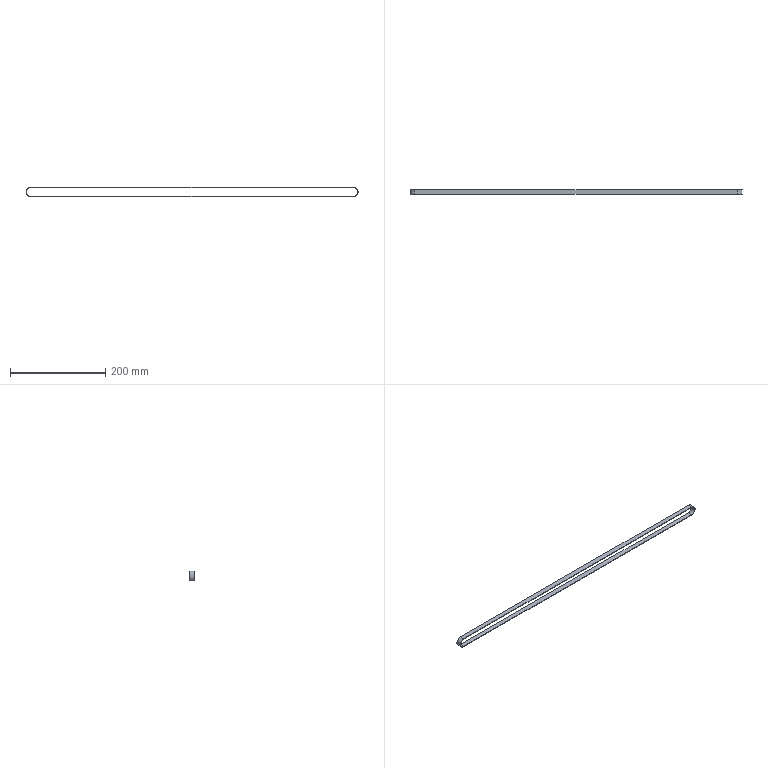Part | SolidWorks | features BaseBody 1 | 1 solid | 10 faces | box 695.6 x 10 x 20.6 mm | volume 16931 mm3 | plane 6 | cylinder 4 | commonest cylinder face diameters 18.2 x2 20.6 x2
STEP:
#1=CARTESIAN_POINT('',(675.,0.,-9.1));
#2=VERTEX_POINT('',#1);
#3=CARTESIAN_POINT('',(0.,0.,-9.1));
#4=VERTEX_POINT('',#3);
#5=CARTESIAN_POINT('',(675.,0.,-9.1));
#6=DIRECTION('',(-1.,0.,0.));
#7=VECTOR('',#6,1000.);
#8=LINE('',#5,#7);
#9=EDGE_CURVE('',#2,#4,#8,.T.);
#10=ORIENTED_EDGE('',*,*,#9,.F.);
#11=CARTESIAN_POINT('',(675.,10.,-9.1));
#12=VERTEX_POINT('',#11);
#13=CARTESIAN_POINT('',(675.,10.,-9.1));
#14=DIRECTION('',(0.,-1.,0.));
#15=VECTOR('',#14,1000.);
#16=LINE('',#13,#15);
#17=EDGE_CURVE('',#12,#2,#16,.T.);
#18=ORIENTED_EDGE('',*,*,#17,.F.);
#19=CARTESIAN_POINT('',(0.,10.,-9.1));
#20=VERTEX_POINT('',#19);
#21=CARTESIAN_POINT('',(675.,10.,-9.1));
#22=DIRECTION('',(-1.,0.,0.));
#23=VECTOR('',#22,1000.);
#24=LINE('',#21,#23);
#25=EDGE_CURVE('',#12,#20,#24,.T.);
#26=ORIENTED_EDGE('',*,*,#25,.T.);
#27=CARTESIAN_POINT('',(0.,10.,-9.1));
#28=DIRECTION('',(0.,-1.,0.));
#29=VECTOR('',#28,1000.);
#30=LINE('',#27,#29);
#31=EDGE_CURVE('',#20,#4,#30,.T.);
#32=ORIENTED_EDGE('',*,*,#31,.T.);
#33=EDGE_LOOP('',(#10,#18,#26,#32));
#34=FACE_OUTER_BOUND('',#33,.T.);
#35=CARTESIAN_POINT('',(675.,10.,-9.1));
#36=DIRECTION('',(0.,0.,1.));
#37=DIRECTION('',(1.,0.,0.));
#38=AXIS2_PLACEMENT_3D('',#35,#36,#37);
#39=PLANE('',#38);
#40=ADVANCED_FACE('',(#34),#39,.T.);
#41=CARTESIAN_POINT('',(675.,0.,9.1));
#42=VERTEX_POINT('',#41);
#43=CARTESIAN_POINT('',(675.,0.,0.));
#44=DIRECTION('',(0.,1.,0.));
#45=DIRECTION('',(0.,0.,1.));
#46=AXIS2_PLACEMENT_3D('',#43,#44,#45);
#47=CIRCLE('',#46,9.1);
#48=EDGE_CURVE('',#42,#2,#47,.T.);
#49=ORIENTED_EDGE('',*,*,#48,.F.);
#50=CARTESIAN_POINT('',(675.,10.,9.1));
#51=VERTEX_POINT('',#50);
#52=CARTESIAN_POINT('',(675.,10.,9.1));
#53=DIRECTION('',(0.,-1.,0.));
#54=VECTOR('',#53,1000.);
#55=LINE('',#52,#54);
#56=EDGE_CURVE('',#51,#42,#55,.T.);
#57=ORIENTED_EDGE('',*,*,#56,.F.);
#58=CARTESIAN_POINT('',(675.,10.,0.));
#59=DIRECTION('',(0.,1.,0.));
#60=DIRECTION('',(0.,0.,1.));
#61=AXIS2_PLACEMENT_3D('',#58,#59,#60);
#62=CIRCLE('',#61,9.1);
#63=EDGE_CURVE('',#51,#12,#62,.T.);
#64=ORIENTED_EDGE('',*,*,#63,.T.);
#65=ORIENTED_EDGE('',*,*,#17,.T.);
#66=EDGE_LOOP('',(#49,#57,#64,#65));
#67=FACE_OUTER_BOUND('',#66,.T.);
#68=CARTESIAN_POINT('',(675.,10.,0.));
#69=DIRECTION('',(0.,-1.,0.));
#70=DIRECTION('',(0.,0.,-1.));
#71=AXIS2_PLACEMENT_3D('',#68,#69,#70);
#72=CYLINDRICAL_SURFACE('',#71,9.1);
#73=ADVANCED_FACE('',(#67),#72,.F.);
#74=CARTESIAN_POINT('',(0.,0.,9.1));
#75=VERTEX_POINT('',#74);
#76=CARTESIAN_POINT('',(0.,0.,9.1));
#77=DIRECTION('',(1.,0.,0.));
#78=VECTOR('',#77,1000.);
#79=LINE('',#76,#78);
#80=EDGE_CURVE('',#75,#42,#79,.T.);
#81=ORIENTED_EDGE('',*,*,#80,.F.);
#82=CARTESIAN_POINT('',(0.,10.,9.1));
#83=VERTEX_POINT('',#82);
#84=CARTESIAN_POINT('',(0.,10.,9.1));
#85=DIRECTION('',(0.,-1.,0.));
#86=VECTOR('',#85,1000.);
#87=LINE('',#84,#86);
#88=EDGE_CURVE('',#83,#75,#87,.T.);
#89=ORIENTED_EDGE('',*,*,#88,.F.);
#90=CARTESIAN_POINT('',(0.,10.,9.1));
#91=DIRECTION('',(1.,0.,0.));
#92=VECTOR('',#91,1000.);
#93=LINE('',#90,#92);
#94=EDGE_CURVE('',#83,#51,#93,.T.);
#95=ORIENTED_EDGE('',*,*,#94,.T.);
#96=ORIENTED_EDGE('',*,*,#56,.T.);
#97=EDGE_LOOP('',(#81,#89,#95,#96));
#98=FACE_OUTER_BOUND('',#97,.T.);
#99=CARTESIAN_POINT('',(0.,10.,9.1));
#100=DIRECTION('',(0.,0.,-1.));
#101=DIRECTION('',(0.,-1.,0.));
#102=AXIS2_PLACEMENT_3D('',#99,#100,#101);
#103=PLANE('',#102);
#104=ADVANCED_FACE('',(#98),#103,.T.);
#105=CARTESIAN_POINT('',(0.,0.,0.));
#106=DIRECTION('',(0.,1.,0.));
#107=DIRECTION('',(0.,0.,1.));
#108=AXIS2_PLACEMENT_3D('',#105,#106,#107);
#109=CIRCLE('',#108,9.1);
#110=EDGE_CURVE('',#4,#75,#109,.T.);
#111=ORIENTED_EDGE('',*,*,#110,.F.);
#112=ORIENTED_EDGE('',*,*,#31,.F.);
#113=CARTESIAN_POINT('',(0.,10.,0.));
#114=DIRECTION('',(0.,1.,0.));
#115=DIRECTION('',(0.,0.,1.));
#116=AXIS2_PLACEMENT_3D('',#113,#114,#115);
#117=CIRCLE('',#116,9.1);
#118=EDGE_CURVE('',#20,#83,#117,.T.);
#119=ORIENTED_EDGE('',*,*,#118,.T.);
#120=ORIENTED_EDGE('',*,*,#88,.T.);
#121=EDGE_LOOP('',(#111,#112,#119,#120));
#122=FACE_OUTER_BOUND('',#121,.T.);
#123=CARTESIAN_POINT('',(0.,10.,0.));
#124=DIRECTION('',(0.,-1.,0.));
#125=DIRECTION('',(0.,0.,-1.));
#126=AXIS2_PLACEMENT_3D('',#123,#124,#125);
#127=CYLINDRICAL_SURFACE('',#126,9.1);
#128=ADVANCED_FACE('',(#122),#127,.F.);
#129=CARTESIAN_POINT('',(675.,0.,-10.3));
#130=VERTEX_POINT('',#129);
#131=CARTESIAN_POINT('',(0.,0.,-10.3));
#132=VERTEX_POINT('',#131);
#133=CARTESIAN_POINT('',(675.,0.,-10.3));
#134=DIRECTION('',(-1.,0.,0.));
#135=VECTOR('',#134,1000.);
#136=LINE('',#133,#135);
#137=EDGE_CURVE('',#130,#132,#136,.T.);
#138=ORIENTED_EDGE('',*,*,#137,.T.);
#139=CARTESIAN_POINT('',(0.,10.,-10.3));
#140=VERTEX_POINT('',#139);
#141=CARTESIAN_POINT('',(0.,10.,-10.3));
#142=DIRECTION('',(0.,-1.,0.));
#143=VECTOR('',#142,1000.);
#144=LINE('',#141,#143);
#145=EDGE_CURVE('',#140,#132,#144,.T.);
#146=ORIENTED_EDGE('',*,*,#145,.F.);
#147=CARTESIAN_POINT('',(675.,10.,-10.3));
#148=VERTEX_POINT('',#147);
#149=CARTESIAN_POINT('',(675.,10.,-10.3));
#150=DIRECTION('',(-1.,0.,0.));
#151=VECTOR('',#150,1000.);
#152=LINE('',#149,#151);
#153=EDGE_CURVE('',#148,#140,#152,.T.);
#154=ORIENTED_EDGE('',*,*,#153,.F.);
#155=CARTESIAN_POINT('',(675.,10.,-10.3));
#156=DIRECTION('',(0.,-1.,0.));
#157=VECTOR('',#156,1000.);
#158=LINE('',#155,#157);
#159=EDGE_CURVE('',#148,#130,#158,.T.);
#160=ORIENTED_EDGE('',*,*,#159,.T.);
#161=EDGE_LOOP('',(#138,#146,#154,#160));
#162=FACE_OUTER_BOUND('',#161,.T.);
#163=CARTESIAN_POINT('',(675.,10.,-10.3));
#164=DIRECTION('',(0.,0.,1.));
#165=DIRECTION('',(1.,0.,0.));
#166=AXIS2_PLACEMENT_3D('',#163,#164,#165);
#167=PLANE('',#166);
#168=ADVANCED_FACE('',(#162),#167,.F.);
#169=CARTESIAN_POINT('',(675.,0.,10.3));
#170=VERTEX_POINT('',#169);
#171=CARTESIAN_POINT('',(675.,0.,0.));
#172=DIRECTION('',(0.,1.,0.));
#173=DIRECTION('',(0.,0.,1.));
#174=AXIS2_PLACEMENT_3D('',#171,#172,#173);
#175=CIRCLE('',#174,10.3);
#176=EDGE_CURVE('',#170,#130,#175,.T.);
#177=ORIENTED_EDGE('',*,*,#176,.T.);
#178=ORIENTED_EDGE('',*,*,#159,.F.);
#179=CARTESIAN_POINT('',(675.,10.,10.3));
#180=VERTEX_POINT('',#179);
#181=CARTESIAN_POINT('',(675.,10.,0.));
#182=DIRECTION('',(0.,1.,0.));
#183=DIRECTION('',(0.,0.,1.));
#184=AXIS2_PLACEMENT_3D('',#181,#182,#183);
#185=CIRCLE('',#184,10.3);
#186=EDGE_CURVE('',#180,#148,#185,.T.);
#187=ORIENTED_EDGE('',*,*,#186,.F.);
#188=CARTESIAN_POINT('',(675.,10.,10.3));
#189=DIRECTION('',(0.,-1.,0.));
#190=VECTOR('',#189,1000.);
#191=LINE('',#188,#190);
#192=EDGE_CURVE('',#180,#170,#191,.T.);
#193=ORIENTED_EDGE('',*,*,#192,.T.);
#194=EDGE_LOOP('',(#177,#178,#187,#193));
#195=FACE_OUTER_BOUND('',#194,.T.);
#196=CARTESIAN_POINT('',(675.,10.,0.));
#197=DIRECTION('',(0.,-1.,0.));
#198=DIRECTION('',(0.,0.,-1.));
#199=AXIS2_PLACEMENT_3D('',#196,#197,#198);
#200=CYLINDRICAL_SURFACE('',#199,10.3);
#201=ADVANCED_FACE('',(#195),#200,.T.);
#202=CARTESIAN_POINT('',(0.,0.,10.3));
#203=VERTEX_POINT('',#202);
#204=CARTESIAN_POINT('',(0.,0.,10.3));
#205=DIRECTION('',(1.,0.,0.));
#206=VECTOR('',#205,1000.);
#207=LINE('',#204,#206);
#208=EDGE_CURVE('',#203,#170,#207,.T.);
#209=ORIENTED_EDGE('',*,*,#208,.T.);
#210=ORIENTED_EDGE('',*,*,#192,.F.);
#211=CARTESIAN_POINT('',(0.,10.,10.3));
#212=VERTEX_POINT('',#211);
#213=CARTESIAN_POINT('',(0.,10.,10.3));
#214=DIRECTION('',(1.,0.,0.));
#215=VECTOR('',#214,1000.);
#216=LINE('',#213,#215);
#217=EDGE_CURVE('',#212,#180,#216,.T.);
#218=ORIENTED_EDGE('',*,*,#217,.F.);
#219=CARTESIAN_POINT('',(0.,10.,10.3));
#220=DIRECTION('',(0.,-1.,0.));
#221=VECTOR('',#220,1000.);
#222=LINE('',#219,#221);
#223=EDGE_CURVE('',#212,#203,#222,.T.);
#224=ORIENTED_EDGE('',*,*,#223,.T.);
#225=EDGE_LOOP('',(#209,#210,#218,#224));
#226=FACE_OUTER_BOUND('',#225,.T.);
#227=CARTESIAN_POINT('',(0.,10.,10.3));
#228=DIRECTION('',(0.,0.,-1.));
#229=DIRECTION('',(0.,-1.,0.));
#230=AXIS2_PLACEMENT_3D('',#227,#228,#229);
#231=PLANE('',#230);
#232=ADVANCED_FACE('',(#226),#231,.F.);
#233=CARTESIAN_POINT('',(0.,0.,0.));
#234=DIRECTION('',(0.,1.,0.));
#235=DIRECTION('',(0.,0.,1.));
#236=AXIS2_PLACEMENT_3D('',#233,#234,#235);
#237=CIRCLE('',#236,10.3);
#238=EDGE_CURVE('',#132,#203,#237,.T.);
#239=ORIENTED_EDGE('',*,*,#238,.T.);
#240=ORIENTED_EDGE('',*,*,#223,.F.);
#241=CARTESIAN_POINT('',(0.,10.,0.));
#242=DIRECTION('',(0.,1.,0.));
#243=DIRECTION('',(0.,0.,1.));
#244=AXIS2_PLACEMENT_3D('',#241,#242,#243);
#245=CIRCLE('',#244,10.3);
#246=EDGE_CURVE('',#140,#212,#245,.T.);
#247=ORIENTED_EDGE('',*,*,#246,.F.);
#248=ORIENTED_EDGE('',*,*,#145,.T.);
#249=EDGE_LOOP('',(#239,#240,#247,#248));
#250=FACE_OUTER_BOUND('',#249,.T.);
#251=CARTESIAN_POINT('',(0.,10.,0.));
#252=DIRECTION('',(0.,-1.,0.));
#253=DIRECTION('',(0.,0.,-1.));
#254=AXIS2_PLACEMENT_3D('',#251,#252,#253);
#255=CYLINDRICAL_SURFACE('',#254,10.3);
#256=ADVANCED_FACE('',(#250),#255,.T.);
#257=ORIENTED_EDGE('',*,*,#110,.T.);
#258=ORIENTED_EDGE('',*,*,#80,.T.);
#259=ORIENTED_EDGE('',*,*,#48,.T.);
#260=ORIENTED_EDGE('',*,*,#9,.T.);
#261=EDGE_LOOP('',(#257,#258,#259,#260));
#262=FACE_BOUND('',#261,.T.);
#263=ORIENTED_EDGE('',*,*,#238,.F.);
#264=ORIENTED_EDGE('',*,*,#137,.F.);
#265=ORIENTED_EDGE('',*,*,#176,.F.);
#266=ORIENTED_EDGE('',*,*,#208,.F.);
#267=EDGE_LOOP('',(#263,#264,#265,#266));
#268=FACE_OUTER_BOUND('',#267,.T.);
#269=CARTESIAN_POINT('',(0.,0.,0.));
#270=DIRECTION('',(0.,1.,0.));
#271=DIRECTION('',(1.,0.,0.));
#272=AXIS2_PLACEMENT_3D('',#269,#270,#271);
#273=PLANE('',#272);
#274=ADVANCED_FACE('',(#262,#268),#273,.F.);
#275=ORIENTED_EDGE('',*,*,#94,.F.);
#276=ORIENTED_EDGE('',*,*,#118,.F.);
#277=ORIENTED_EDGE('',*,*,#25,.F.);
#278=ORIENTED_EDGE('',*,*,#63,.F.);
#279=EDGE_LOOP('',(#275,#276,#277,#278));
#280=FACE_BOUND('',#279,.T.);
#281=ORIENTED_EDGE('',*,*,#246,.T.);
#282=ORIENTED_EDGE('',*,*,#217,.T.);
#283=ORIENTED_EDGE('',*,*,#186,.T.);
#284=ORIENTED_EDGE('',*,*,#153,.T.);
#285=EDGE_LOOP('',(#281,#282,#283,#284));
#286=FACE_OUTER_BOUND('',#285,.T.);
#287=CARTESIAN_POINT('',(0.,10.,0.));
#288=DIRECTION('',(0.,1.,0.));
#289=DIRECTION('',(1.,0.,0.));
#290=AXIS2_PLACEMENT_3D('',#287,#288,#289);
#291=PLANE('',#290);
#292=ADVANCED_FACE('',(#280,#286),#291,.T.);
#293=CLOSED_SHELL('',(#40,#73,#104,#128,#168,#201,#232,#256,#274,#292));
#294=MANIFOLD_SOLID_BREP('',#293);
#295=CARTESIAN_POINT('',(0.,0.,0.));
#296=DIRECTION('',(0.,0.,1.));
#297=DIRECTION('',(1.,0.,0.));
#298=AXIS2_PLACEMENT_3D('',#295,#296,#297);
#299=(LENGTH_UNIT()NAMED_UNIT(*)SI_UNIT(.MILLI.,.METRE.));
#300=UNCERTAINTY_MEASURE_WITH_UNIT(LENGTH_MEASURE(0.00001),#299,'','');
#301=(NAMED_UNIT(*)PLANE_ANGLE_UNIT()SI_UNIT($,.RADIAN.));
#302=(NAMED_UNIT(*)SI_UNIT($,.STERADIAN.)SOLID_ANGLE_UNIT());
#303=(GEOMETRIC_REPRESENTATION_CONTEXT(3)GLOBAL_UNCERTAINTY_ASSIGNED_CONTEXT((#300))GLOBAL_UNIT_ASSIGNED_CONTEXT((#299,#301,#302))REPRESENTATION_CONTEXT('',''));
#304=ADVANCED_BREP_SHAPE_REPRESENTATION('',(#294,#298),#303);